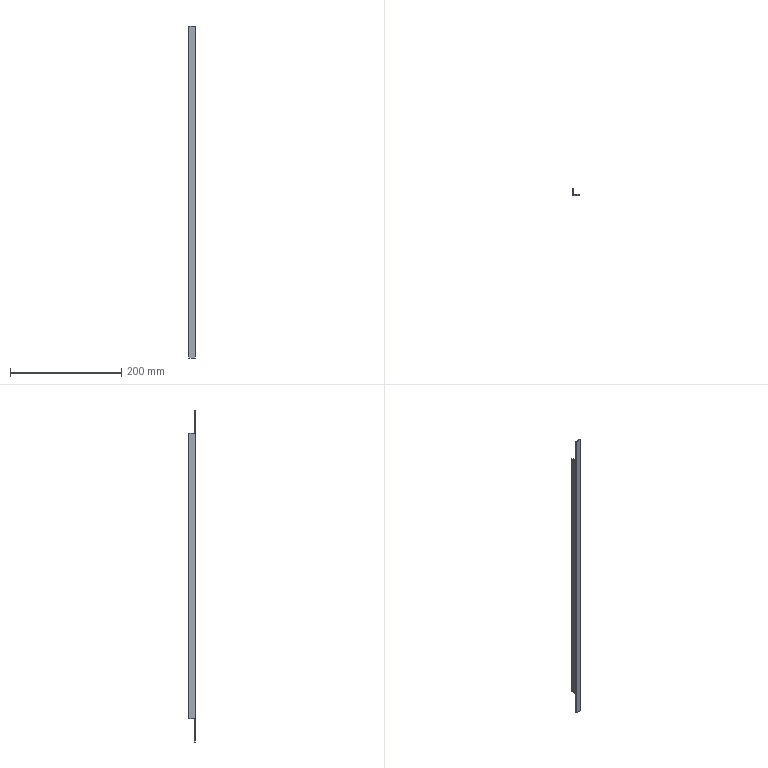Part | SolidWorks | features BaseBody 1 | 1 solid | 20 faces | box 12 x 12 x 597.2 mm | volume 15203 mm3 | plane 14 | cylinder 6 | commonest cylinder face diameters 0.6 x4 1 x2
STEP:
#1=CARTESIAN_POINT('',(0.5,0.,298.6));
#2=VERTEX_POINT('',#1);
#3=CARTESIAN_POINT('',(0.5,0.,-298.6));
#4=VERTEX_POINT('',#3);
#5=CARTESIAN_POINT('',(0.5,0.,0.));
#6=DIRECTION('',(0.,0.,-1.));
#7=VECTOR('',#6,1000.);
#8=LINE('',#5,#7);
#9=EDGE_CURVE('',#2,#4,#8,.T.);
#10=ORIENTED_EDGE('',*,*,#9,.F.);
#11=CARTESIAN_POINT('',(0.,0.5,298.6));
#12=VERTEX_POINT('',#11);
#13=CARTESIAN_POINT('',(0.5,0.5,298.6));
#14=DIRECTION('',(0.,0.,-1.));
#15=DIRECTION('',(0.,1.,0.));
#16=AXIS2_PLACEMENT_3D('',#13,#14,#15);
#17=CIRCLE('',#16,0.5);
#18=EDGE_CURVE('',#2,#12,#17,.T.);
#19=ORIENTED_EDGE('',*,*,#18,.T.);
#20=CARTESIAN_POINT('',(0.,0.5,-298.6));
#21=VERTEX_POINT('',#20);
#22=CARTESIAN_POINT('',(0.,0.5,0.));
#23=DIRECTION('',(0.,0.,1.));
#24=VECTOR('',#23,1000.);
#25=LINE('',#22,#24);
#26=EDGE_CURVE('',#21,#12,#25,.T.);
#27=ORIENTED_EDGE('',*,*,#26,.F.);
#28=CARTESIAN_POINT('',(0.5,0.5,-298.6));
#29=DIRECTION('',(0.,0.,-1.));
#30=DIRECTION('',(0.,1.,0.));
#31=AXIS2_PLACEMENT_3D('',#28,#29,#30);
#32=CIRCLE('',#31,0.5);
#33=EDGE_CURVE('',#4,#21,#32,.T.);
#34=ORIENTED_EDGE('',*,*,#33,.F.);
#35=EDGE_LOOP('',(#10,#19,#27,#34));
#36=FACE_OUTER_BOUND('',#35,.T.);
#37=CARTESIAN_POINT('',(0.5,0.5,298.6));
#38=DIRECTION('',(0.,0.,-1.));
#39=DIRECTION('',(0.,1.,0.));
#40=AXIS2_PLACEMENT_3D('',#37,#38,#39);
#41=CYLINDRICAL_SURFACE('',#40,0.5);
#42=ADVANCED_FACE('',(#36),#41,.T.);
#43=CARTESIAN_POINT('',(11.7,0.,298.6));
#44=VERTEX_POINT('',#43);
#45=CARTESIAN_POINT('',(11.7,0.,-298.6));
#46=VERTEX_POINT('',#45);
#47=CARTESIAN_POINT('',(11.7,0.,0.));
#48=DIRECTION('',(0.,0.,-1.));
#49=VECTOR('',#48,1000.);
#50=LINE('',#47,#49);
#51=EDGE_CURVE('',#44,#46,#50,.T.);
#52=ORIENTED_EDGE('',*,*,#51,.F.);
#53=CARTESIAN_POINT('',(6.1,0.,298.6));
#54=DIRECTION('',(1.,0.,0.));
#55=VECTOR('',#54,1000.);
#56=LINE('',#53,#55);
#57=EDGE_CURVE('',#2,#44,#56,.T.);
#58=ORIENTED_EDGE('',*,*,#57,.F.);
#59=ORIENTED_EDGE('',*,*,#9,.T.);
#60=CARTESIAN_POINT('',(6.1,0.,-298.6));
#61=DIRECTION('',(-1.,0.,0.));
#62=VECTOR('',#61,1000.);
#63=LINE('',#60,#62);
#64=EDGE_CURVE('',#46,#4,#63,.T.);
#65=ORIENTED_EDGE('',*,*,#64,.F.);
#66=EDGE_LOOP('',(#52,#58,#59,#65));
#67=FACE_OUTER_BOUND('',#66,.T.);
#68=CARTESIAN_POINT('',(0.5,0.,-298.6));
#69=DIRECTION('',(0.,1.,0.));
#70=DIRECTION('',(0.,0.,1.));
#71=AXIS2_PLACEMENT_3D('',#68,#69,#70);
#72=PLANE('',#71);
#73=ADVANCED_FACE('',(#67),#72,.F.);
#74=CARTESIAN_POINT('',(0.,1.2,-298.6));
#75=VERTEX_POINT('',#74);
#76=CARTESIAN_POINT('',(0.,1.2,-256.4));
#77=VERTEX_POINT('',#76);
#78=CARTESIAN_POINT('',(0.,1.2,0.));
#79=DIRECTION('',(0.,0.,1.));
#80=VECTOR('',#79,1000.);
#81=LINE('',#78,#80);
#82=EDGE_CURVE('',#75,#77,#81,.T.);
#83=ORIENTED_EDGE('',*,*,#82,.F.);
#84=CARTESIAN_POINT('',(0.,6.1,-298.6));
#85=DIRECTION('',(0.,1.,0.));
#86=VECTOR('',#85,1000.);
#87=LINE('',#84,#86);
#88=EDGE_CURVE('',#21,#75,#87,.T.);
#89=ORIENTED_EDGE('',*,*,#88,.F.);
#90=ORIENTED_EDGE('',*,*,#26,.T.);
#91=CARTESIAN_POINT('',(0.,1.2,298.6));
#92=VERTEX_POINT('',#91);
#93=CARTESIAN_POINT('',(0.,6.1,298.6));
#94=DIRECTION('',(0.,-1.,0.));
#95=VECTOR('',#94,1000.);
#96=LINE('',#93,#95);
#97=EDGE_CURVE('',#92,#12,#96,.T.);
#98=ORIENTED_EDGE('',*,*,#97,.F.);
#99=CARTESIAN_POINT('',(0.,1.2,256.4));
#100=VERTEX_POINT('',#99);
#101=CARTESIAN_POINT('',(0.,1.2,0.));
#102=DIRECTION('',(0.,0.,1.));
#103=VECTOR('',#102,1000.);
#104=LINE('',#101,#103);
#105=EDGE_CURVE('',#100,#92,#104,.T.);
#106=ORIENTED_EDGE('',*,*,#105,.F.);
#107=CARTESIAN_POINT('',(0.,11.7,256.4));
#108=VERTEX_POINT('',#107);
#109=CARTESIAN_POINT('',(0.,6.1,256.4));
#110=DIRECTION('',(0.,-1.,0.));
#111=VECTOR('',#110,1000.);
#112=LINE('',#109,#111);
#113=EDGE_CURVE('',#108,#100,#112,.T.);
#114=ORIENTED_EDGE('',*,*,#113,.F.);
#115=CARTESIAN_POINT('',(0.,11.7,-256.4));
#116=VERTEX_POINT('',#115);
#117=CARTESIAN_POINT('',(0.,11.7,0.));
#118=DIRECTION('',(0.,0.,1.));
#119=VECTOR('',#118,1000.);
#120=LINE('',#117,#119);
#121=EDGE_CURVE('',#116,#108,#120,.T.);
#122=ORIENTED_EDGE('',*,*,#121,.F.);
#123=CARTESIAN_POINT('',(0.,6.1,-256.4));
#124=DIRECTION('',(0.,1.,0.));
#125=VECTOR('',#124,1000.);
#126=LINE('',#123,#125);
#127=EDGE_CURVE('',#77,#116,#126,.T.);
#128=ORIENTED_EDGE('',*,*,#127,.F.);
#129=EDGE_LOOP('',(#83,#89,#90,#98,#106,#114,#122,#128));
#130=FACE_OUTER_BOUND('',#129,.T.);
#131=CARTESIAN_POINT('',(0.,0.5,298.6));
#132=DIRECTION('',(1.,0.,0.));
#133=DIRECTION('',(0.,0.,-1.));
#134=AXIS2_PLACEMENT_3D('',#131,#132,#133);
#135=PLANE('',#134);
#136=ADVANCED_FACE('',(#130),#135,.F.);
#137=ORIENTED_EDGE('',*,*,#33,.T.);
#138=ORIENTED_EDGE('',*,*,#88,.T.);
#139=CARTESIAN_POINT('',(1.2,1.2,-298.6));
#140=VERTEX_POINT('',#139);
#141=CARTESIAN_POINT('',(6.,1.2,-298.6));
#142=DIRECTION('',(1.,0.,0.));
#143=VECTOR('',#142,1000.);
#144=LINE('',#141,#143);
#145=EDGE_CURVE('',#75,#140,#144,.T.);
#146=ORIENTED_EDGE('',*,*,#145,.T.);
#147=CARTESIAN_POINT('',(1.2,1.7,-298.6));
#148=VERTEX_POINT('',#147);
#149=CARTESIAN_POINT('',(1.2,1.45,-298.6));
#150=DIRECTION('',(0.,1.,0.));
#151=VECTOR('',#150,1000.);
#152=LINE('',#149,#151);
#153=EDGE_CURVE('',#140,#148,#152,.T.);
#154=ORIENTED_EDGE('',*,*,#153,.T.);
#155=CARTESIAN_POINT('',(1.7,1.2,-298.6));
#156=VERTEX_POINT('',#155);
#157=CARTESIAN_POINT('',(1.7,1.7,-298.6));
#158=DIRECTION('',(0.,0.,-1.));
#159=DIRECTION('',(0.,1.,0.));
#160=AXIS2_PLACEMENT_3D('',#157,#158,#159);
#161=CIRCLE('',#160,0.5);
#162=EDGE_CURVE('',#156,#148,#161,.T.);
#163=ORIENTED_EDGE('',*,*,#162,.F.);
#164=CARTESIAN_POINT('',(11.7,1.2,-298.6));
#165=VERTEX_POINT('',#164);
#166=CARTESIAN_POINT('',(6.,1.2,-298.6));
#167=DIRECTION('',(1.,0.,0.));
#168=VECTOR('',#167,1000.);
#169=LINE('',#166,#168);
#170=EDGE_CURVE('',#156,#165,#169,.T.);
#171=ORIENTED_EDGE('',*,*,#170,.T.);
#172=CARTESIAN_POINT('',(12.,0.9,-298.6));
#173=VERTEX_POINT('',#172);
#174=CARTESIAN_POINT('',(11.7,0.9,-298.6));
#175=DIRECTION('',(0.,0.,-1.));
#176=DIRECTION('',(0.,1.,0.));
#177=AXIS2_PLACEMENT_3D('',#174,#175,#176);
#178=CIRCLE('',#177,0.3);
#179=EDGE_CURVE('',#165,#173,#178,.T.);
#180=ORIENTED_EDGE('',*,*,#179,.T.);
#181=CARTESIAN_POINT('',(12.,0.3,-298.6));
#182=VERTEX_POINT('',#181);
#183=CARTESIAN_POINT('',(12.,0.6,-298.6));
#184=DIRECTION('',(0.,-1.,0.));
#185=VECTOR('',#184,1000.);
#186=LINE('',#183,#185);
#187=EDGE_CURVE('',#173,#182,#186,.T.);
#188=ORIENTED_EDGE('',*,*,#187,.T.);
#189=CARTESIAN_POINT('',(11.7,0.3,-298.6));
#190=DIRECTION('',(0.,0.,-1.));
#191=DIRECTION('',(0.,1.,0.));
#192=AXIS2_PLACEMENT_3D('',#189,#190,#191);
#193=CIRCLE('',#192,0.3);
#194=EDGE_CURVE('',#182,#46,#193,.T.);
#195=ORIENTED_EDGE('',*,*,#194,.T.);
#196=ORIENTED_EDGE('',*,*,#64,.T.);
#197=EDGE_LOOP('',(#137,#138,#146,#154,#163,#171,#180,#188,#195,#196));
#198=FACE_OUTER_BOUND('',#197,.T.);
#199=CARTESIAN_POINT('',(12.,0.,-298.6));
#200=DIRECTION('',(0.,0.,-1.));
#201=DIRECTION('',(-1.,0.,0.));
#202=AXIS2_PLACEMENT_3D('',#199,#200,#201);
#203=PLANE('',#202);
#204=ADVANCED_FACE('',(#198),#203,.T.);
#205=CARTESIAN_POINT('',(12.,0.3,298.6));
#206=VERTEX_POINT('',#205);
#207=CARTESIAN_POINT('',(12.,0.3,0.));
#208=DIRECTION('',(0.,0.,-1.));
#209=VECTOR('',#208,1000.);
#210=LINE('',#207,#209);
#211=EDGE_CURVE('',#206,#182,#210,.T.);
#212=ORIENTED_EDGE('',*,*,#211,.F.);
#213=CARTESIAN_POINT('',(11.7,0.3,298.6));
#214=DIRECTION('',(0.,0.,1.));
#215=DIRECTION('',(0.,1.,0.));
#216=AXIS2_PLACEMENT_3D('',#213,#214,#215);
#217=CIRCLE('',#216,0.3);
#218=EDGE_CURVE('',#44,#206,#217,.T.);
#219=ORIENTED_EDGE('',*,*,#218,.F.);
#220=ORIENTED_EDGE('',*,*,#51,.T.);
#221=ORIENTED_EDGE('',*,*,#194,.F.);
#222=EDGE_LOOP('',(#212,#219,#220,#221));
#223=FACE_OUTER_BOUND('',#222,.T.);
#224=CARTESIAN_POINT('',(11.7,0.3,298.6));
#225=DIRECTION('',(0.,0.,-1.));
#226=DIRECTION('',(0.,1.,0.));
#227=AXIS2_PLACEMENT_3D('',#224,#225,#226);
#228=CYLINDRICAL_SURFACE('',#227,0.3);
#229=ADVANCED_FACE('',(#223),#228,.T.);
#230=CARTESIAN_POINT('',(1.2,1.2,298.6));
#231=VERTEX_POINT('',#230);
#232=CARTESIAN_POINT('',(6.,1.2,298.6));
#233=DIRECTION('',(1.,0.,0.));
#234=VECTOR('',#233,1000.);
#235=LINE('',#232,#234);
#236=EDGE_CURVE('',#92,#231,#235,.T.);
#237=ORIENTED_EDGE('',*,*,#236,.F.);
#238=ORIENTED_EDGE('',*,*,#97,.T.);
#239=ORIENTED_EDGE('',*,*,#18,.F.);
#240=ORIENTED_EDGE('',*,*,#57,.T.);
#241=ORIENTED_EDGE('',*,*,#218,.T.);
#242=CARTESIAN_POINT('',(12.,0.9,298.6));
#243=VERTEX_POINT('',#242);
#244=CARTESIAN_POINT('',(12.,0.8551,298.6));
#245=DIRECTION('',(0.,-1.,0.));
#246=VECTOR('',#245,1000.);
#247=LINE('',#244,#246);
#248=EDGE_CURVE('',#243,#206,#247,.T.);
#249=ORIENTED_EDGE('',*,*,#248,.F.);
#250=CARTESIAN_POINT('',(11.7,1.2,298.6));
#251=VERTEX_POINT('',#250);
#252=CARTESIAN_POINT('',(11.7,0.9,298.6));
#253=DIRECTION('',(0.,0.,1.));
#254=DIRECTION('',(0.,1.,0.));
#255=AXIS2_PLACEMENT_3D('',#252,#253,#254);
#256=CIRCLE('',#255,0.3);
#257=EDGE_CURVE('',#243,#251,#256,.T.);
#258=ORIENTED_EDGE('',*,*,#257,.T.);
#259=CARTESIAN_POINT('',(1.7,1.2,298.6));
#260=VERTEX_POINT('',#259);
#261=CARTESIAN_POINT('',(6.,1.2,298.6));
#262=DIRECTION('',(1.,0.,0.));
#263=VECTOR('',#262,1000.);
#264=LINE('',#261,#263);
#265=EDGE_CURVE('',#260,#251,#264,.T.);
#266=ORIENTED_EDGE('',*,*,#265,.F.);
#267=CARTESIAN_POINT('',(1.2,1.7,298.6));
#268=VERTEX_POINT('',#267);
#269=CARTESIAN_POINT('',(1.7,1.7,298.6));
#270=DIRECTION('',(0.,0.,1.));
#271=DIRECTION('',(0.,1.,0.));
#272=AXIS2_PLACEMENT_3D('',#269,#270,#271);
#273=CIRCLE('',#272,0.5);
#274=EDGE_CURVE('',#268,#260,#273,.T.);
#275=ORIENTED_EDGE('',*,*,#274,.F.);
#276=CARTESIAN_POINT('',(1.2,1.45,298.6));
#277=DIRECTION('',(0.,1.,0.));
#278=VECTOR('',#277,1000.);
#279=LINE('',#276,#278);
#280=EDGE_CURVE('',#231,#268,#279,.T.);
#281=ORIENTED_EDGE('',*,*,#280,.F.);
#282=EDGE_LOOP('',(#237,#238,#239,#240,#241,#249,#258,#266,#275,#281));
#283=FACE_OUTER_BOUND('',#282,.T.);
#284=CARTESIAN_POINT('',(12.,0.,298.6));
#285=DIRECTION('',(0.,0.,-1.));
#286=DIRECTION('',(-1.,0.,0.));
#287=AXIS2_PLACEMENT_3D('',#284,#285,#286);
#288=PLANE('',#287);
#289=ADVANCED_FACE('',(#283),#288,.F.);
#290=CARTESIAN_POINT('',(1.2,1.7,-256.4));
#291=VERTEX_POINT('',#290);
#292=CARTESIAN_POINT('',(1.2,1.2,-256.4));
#293=VERTEX_POINT('',#292);
#294=CARTESIAN_POINT('',(1.2,1.45,-256.4));
#295=DIRECTION('',(0.,-1.,0.));
#296=VECTOR('',#295,1000.);
#297=LINE('',#294,#296);
#298=EDGE_CURVE('',#291,#293,#297,.T.);
#299=ORIENTED_EDGE('',*,*,#298,.T.);
#300=CARTESIAN_POINT('',(0.6,1.2,-256.4));
#301=DIRECTION('',(1.,0.,0.));
#302=VECTOR('',#301,1000.);
#303=LINE('',#300,#302);
#304=EDGE_CURVE('',#77,#293,#303,.T.);
#305=ORIENTED_EDGE('',*,*,#304,.F.);
#306=ORIENTED_EDGE('',*,*,#127,.T.);
#307=CARTESIAN_POINT('',(0.3,12.,-256.4));
#308=VERTEX_POINT('',#307);
#309=CARTESIAN_POINT('',(0.3,11.7,-256.4));
#310=DIRECTION('',(0.,0.,1.));
#311=DIRECTION('',(-1.,0.,0.));
#312=AXIS2_PLACEMENT_3D('',#309,#310,#311);
#313=CIRCLE('',#312,0.3);
#314=EDGE_CURVE('',#308,#116,#313,.T.);
#315=ORIENTED_EDGE('',*,*,#314,.F.);
#316=CARTESIAN_POINT('',(0.9,12.,-256.4));
#317=VERTEX_POINT('',#316);
#318=CARTESIAN_POINT('',(0.6,12.,-256.4));
#319=DIRECTION('',(1.,0.,0.));
#320=VECTOR('',#319,1000.);
#321=LINE('',#318,#320);
#322=EDGE_CURVE('',#308,#317,#321,.T.);
#323=ORIENTED_EDGE('',*,*,#322,.T.);
#324=CARTESIAN_POINT('',(1.2,11.7,-256.4));
#325=VERTEX_POINT('',#324);
#326=CARTESIAN_POINT('',(0.9,11.7,-256.4));
#327=DIRECTION('',(0.,0.,-1.));
#328=DIRECTION('',(-1.,0.,0.));
#329=AXIS2_PLACEMENT_3D('',#326,#327,#328);
#330=CIRCLE('',#329,0.3);
#331=EDGE_CURVE('',#317,#325,#330,.T.);
#332=ORIENTED_EDGE('',*,*,#331,.T.);
#333=CARTESIAN_POINT('',(1.2,6.6,-256.4));
#334=DIRECTION('',(0.,1.,0.));
#335=VECTOR('',#334,1000.);
#336=LINE('',#333,#335);
#337=EDGE_CURVE('',#291,#325,#336,.T.);
#338=ORIENTED_EDGE('',*,*,#337,.F.);
#339=EDGE_LOOP('',(#299,#305,#306,#315,#323,#332,#338));
#340=FACE_OUTER_BOUND('',#339,.T.);
#341=CARTESIAN_POINT('',(0.,1.2,-256.4));
#342=DIRECTION('',(0.,0.,1.));
#343=DIRECTION('',(1.,0.,0.));
#344=AXIS2_PLACEMENT_3D('',#341,#342,#343);
#345=PLANE('',#344);
#346=ADVANCED_FACE('',(#340),#345,.F.);
#347=CARTESIAN_POINT('',(1.2,1.2,-277.5));
#348=DIRECTION('',(0.,0.,1.));
#349=VECTOR('',#348,1000.);
#350=LINE('',#347,#349);
#351=EDGE_CURVE('',#140,#293,#350,.T.);
#352=ORIENTED_EDGE('',*,*,#351,.F.);
#353=ORIENTED_EDGE('',*,*,#145,.F.);
#354=ORIENTED_EDGE('',*,*,#82,.T.);
#355=ORIENTED_EDGE('',*,*,#304,.T.);
#356=EDGE_LOOP('',(#352,#353,#354,#355));
#357=FACE_OUTER_BOUND('',#356,.T.);
#358=CARTESIAN_POINT('',(0.,1.2,-298.6));
#359=DIRECTION('',(0.,-1.,0.));
#360=DIRECTION('',(1.,0.,0.));
#361=AXIS2_PLACEMENT_3D('',#358,#359,#360);
#362=PLANE('',#361);
#363=ADVANCED_FACE('',(#357),#362,.F.);
#364=CARTESIAN_POINT('',(1.2,1.2,256.4));
#365=VERTEX_POINT('',#364);
#366=CARTESIAN_POINT('',(1.2,1.2,277.5));
#367=DIRECTION('',(0.,0.,1.));
#368=VECTOR('',#367,1000.);
#369=LINE('',#366,#368);
#370=EDGE_CURVE('',#365,#231,#369,.T.);
#371=ORIENTED_EDGE('',*,*,#370,.F.);
#372=CARTESIAN_POINT('',(0.6,1.2,256.4));
#373=DIRECTION('',(1.,0.,0.));
#374=VECTOR('',#373,1000.);
#375=LINE('',#372,#374);
#376=EDGE_CURVE('',#100,#365,#375,.T.);
#377=ORIENTED_EDGE('',*,*,#376,.F.);
#378=ORIENTED_EDGE('',*,*,#105,.T.);
#379=ORIENTED_EDGE('',*,*,#236,.T.);
#380=EDGE_LOOP('',(#371,#377,#378,#379));
#381=FACE_OUTER_BOUND('',#380,.T.);
#382=CARTESIAN_POINT('',(0.,1.2,256.4));
#383=DIRECTION('',(0.,-1.,0.));
#384=DIRECTION('',(1.,0.,0.));
#385=AXIS2_PLACEMENT_3D('',#382,#383,#384);
#386=PLANE('',#385);
#387=ADVANCED_FACE('',(#381),#386,.F.);
#388=CARTESIAN_POINT('',(0.3,12.,256.4));
#389=VERTEX_POINT('',#388);
#390=CARTESIAN_POINT('',(0.3,11.7,256.4));
#391=DIRECTION('',(0.,0.,-1.));
#392=DIRECTION('',(-1.,0.,0.));
#393=AXIS2_PLACEMENT_3D('',#390,#391,#392);
#394=CIRCLE('',#393,0.3);
#395=EDGE_CURVE('',#108,#389,#394,.T.);
#396=ORIENTED_EDGE('',*,*,#395,.F.);
#397=ORIENTED_EDGE('',*,*,#113,.T.);
#398=ORIENTED_EDGE('',*,*,#376,.T.);
#399=CARTESIAN_POINT('',(1.2,1.7,256.4));
#400=VERTEX_POINT('',#399);
#401=CARTESIAN_POINT('',(1.2,6.6,256.4));
#402=DIRECTION('',(0.,-1.,0.));
#403=VECTOR('',#402,1000.);
#404=LINE('',#401,#403);
#405=EDGE_CURVE('',#400,#365,#404,.T.);
#406=ORIENTED_EDGE('',*,*,#405,.F.);
#407=CARTESIAN_POINT('',(1.2,11.7,256.4));
#408=VERTEX_POINT('',#407);
#409=CARTESIAN_POINT('',(1.2,6.6,256.4));
#410=DIRECTION('',(0.,-1.,0.));
#411=VECTOR('',#410,1000.);
#412=LINE('',#409,#411);
#413=EDGE_CURVE('',#408,#400,#412,.T.);
#414=ORIENTED_EDGE('',*,*,#413,.F.);
#415=CARTESIAN_POINT('',(0.9,12.,256.4));
#416=VERTEX_POINT('',#415);
#417=CARTESIAN_POINT('',(0.9,11.7,256.4));
#418=DIRECTION('',(0.,0.,1.));
#419=DIRECTION('',(-1.,0.,0.));
#420=AXIS2_PLACEMENT_3D('',#417,#418,#419);
#421=CIRCLE('',#420,0.3);
#422=EDGE_CURVE('',#408,#416,#421,.T.);
#423=ORIENTED_EDGE('',*,*,#422,.T.);
#424=CARTESIAN_POINT('',(0.6,12.,256.4));
#425=DIRECTION('',(-1.,0.,0.));
#426=VECTOR('',#425,1000.);
#427=LINE('',#424,#426);
#428=EDGE_CURVE('',#416,#389,#427,.T.);
#429=ORIENTED_EDGE('',*,*,#428,.T.);
#430=EDGE_LOOP('',(#396,#397,#398,#406,#414,#423,#429));
#431=FACE_OUTER_BOUND('',#430,.T.);
#432=CARTESIAN_POINT('',(1.2,1.2,256.4));
#433=DIRECTION('',(0.,0.,-1.));
#434=DIRECTION('',(-1.,0.,0.));
#435=AXIS2_PLACEMENT_3D('',#432,#433,#434);
#436=PLANE('',#435);
#437=ADVANCED_FACE('',(#431),#436,.F.);
#438=ORIENTED_EDGE('',*,*,#314,.T.);
#439=ORIENTED_EDGE('',*,*,#121,.T.);
#440=ORIENTED_EDGE('',*,*,#395,.T.);
#441=CARTESIAN_POINT('',(0.3,12.,0.));
#442=DIRECTION('',(0.,0.,1.));
#443=VECTOR('',#442,1000.);
#444=LINE('',#441,#443);
#445=EDGE_CURVE('',#308,#389,#444,.T.);
#446=ORIENTED_EDGE('',*,*,#445,.F.);
#447=EDGE_LOOP('',(#438,#439,#440,#446));
#448=FACE_OUTER_BOUND('',#447,.T.);
#449=CARTESIAN_POINT('',(0.3,11.7,256.4));
#450=DIRECTION('',(0.,0.,-1.));
#451=DIRECTION('',(-1.,0.,0.));
#452=AXIS2_PLACEMENT_3D('',#449,#450,#451);
#453=CYLINDRICAL_SURFACE('',#452,0.3);
#454=ADVANCED_FACE('',(#448),#453,.T.);
#455=CARTESIAN_POINT('',(1.7,1.2,0.));
#456=DIRECTION('',(0.,0.,-1.));
#457=VECTOR('',#456,1000.);
#458=LINE('',#455,#457);
#459=EDGE_CURVE('',#260,#156,#458,.T.);
#460=ORIENTED_EDGE('',*,*,#459,.F.);
#461=ORIENTED_EDGE('',*,*,#265,.T.);
#462=CARTESIAN_POINT('',(11.7,1.2,0.));
#463=DIRECTION('',(0.,0.,1.));
#464=VECTOR('',#463,1000.);
#465=LINE('',#462,#464);
#466=EDGE_CURVE('',#165,#251,#465,.T.);
#467=ORIENTED_EDGE('',*,*,#466,.F.);
#468=ORIENTED_EDGE('',*,*,#170,.F.);
#469=EDGE_LOOP('',(#460,#461,#467,#468));
#470=FACE_OUTER_BOUND('',#469,.T.);
#471=CARTESIAN_POINT('',(1.7,1.2,-298.6));
#472=DIRECTION('',(0.,-1.,0.));
#473=DIRECTION('',(1.,0.,0.));
#474=AXIS2_PLACEMENT_3D('',#471,#472,#473);
#475=PLANE('',#474);
#476=ADVANCED_FACE('',(#470),#475,.F.);
#477=CARTESIAN_POINT('',(12.,0.9,0.));
#478=DIRECTION('',(0.,0.,-1.));
#479=VECTOR('',#478,1000.);
#480=LINE('',#477,#479);
#481=EDGE_CURVE('',#243,#173,#480,.T.);
#482=ORIENTED_EDGE('',*,*,#481,.F.);
#483=ORIENTED_EDGE('',*,*,#248,.T.);
#484=ORIENTED_EDGE('',*,*,#211,.T.);
#485=ORIENTED_EDGE('',*,*,#187,.F.);
#486=EDGE_LOOP('',(#482,#483,#484,#485));
#487=FACE_OUTER_BOUND('',#486,.T.);
#488=CARTESIAN_POINT('',(12.,0.3,-298.6));
#489=DIRECTION('',(-1.,0.,0.));
#490=DIRECTION('',(0.,0.,1.));
#491=AXIS2_PLACEMENT_3D('',#488,#489,#490);
#492=PLANE('',#491);
#493=ADVANCED_FACE('',(#487),#492,.F.);
#494=ORIENTED_EDGE('',*,*,#337,.T.);
#495=CARTESIAN_POINT('',(1.2,11.7,0.));
#496=DIRECTION('',(0.,0.,-1.));
#497=VECTOR('',#496,1000.);
#498=LINE('',#495,#497);
#499=EDGE_CURVE('',#408,#325,#498,.T.);
#500=ORIENTED_EDGE('',*,*,#499,.F.);
#501=ORIENTED_EDGE('',*,*,#413,.T.);
#502=CARTESIAN_POINT('',(1.2,1.7,0.));
#503=DIRECTION('',(0.,0.,1.));
#504=VECTOR('',#503,1000.);
#505=LINE('',#502,#504);
#506=EDGE_CURVE('',#291,#400,#505,.T.);
#507=ORIENTED_EDGE('',*,*,#506,.F.);
#508=EDGE_LOOP('',(#494,#500,#501,#507));
#509=FACE_OUTER_BOUND('',#508,.T.);
#510=CARTESIAN_POINT('',(1.2,11.7,-256.4));
#511=DIRECTION('',(-1.,0.,0.));
#512=DIRECTION('',(0.,-1.,0.));
#513=AXIS2_PLACEMENT_3D('',#510,#511,#512);
#514=PLANE('',#513);
#515=ADVANCED_FACE('',(#509),#514,.F.);
#516=ORIENTED_EDGE('',*,*,#351,.T.);
#517=ORIENTED_EDGE('',*,*,#298,.F.);
#518=CARTESIAN_POINT('',(1.2,1.7,-277.5));
#519=DIRECTION('',(0.,0.,1.));
#520=VECTOR('',#519,1000.);
#521=LINE('',#518,#520);
#522=EDGE_CURVE('',#148,#291,#521,.T.);
#523=ORIENTED_EDGE('',*,*,#522,.F.);
#524=ORIENTED_EDGE('',*,*,#153,.F.);
#525=EDGE_LOOP('',(#516,#517,#523,#524));
#526=FACE_OUTER_BOUND('',#525,.T.);
#527=CARTESIAN_POINT('',(1.2,1.2,-298.6));
#528=DIRECTION('',(1.,0.,0.));
#529=DIRECTION('',(0.,1.,0.));
#530=AXIS2_PLACEMENT_3D('',#527,#528,#529);
#531=PLANE('',#530);
#532=ADVANCED_FACE('',(#526),#531,.F.);
#533=ORIENTED_EDGE('',*,*,#280,.T.);
#534=CARTESIAN_POINT('',(1.2,1.7,277.5));
#535=DIRECTION('',(0.,0.,-1.));
#536=VECTOR('',#535,1000.);
#537=LINE('',#534,#536);
#538=EDGE_CURVE('',#268,#400,#537,.T.);
#539=ORIENTED_EDGE('',*,*,#538,.T.);
#540=ORIENTED_EDGE('',*,*,#405,.T.);
#541=ORIENTED_EDGE('',*,*,#370,.T.);
#542=EDGE_LOOP('',(#533,#539,#540,#541));
#543=FACE_OUTER_BOUND('',#542,.T.);
#544=CARTESIAN_POINT('',(1.2,1.7,256.4));
#545=DIRECTION('',(-1.,0.,0.));
#546=DIRECTION('',(0.,-1.,0.));
#547=AXIS2_PLACEMENT_3D('',#544,#545,#546);
#548=PLANE('',#547);
#549=ADVANCED_FACE('',(#543),#548,.T.);
#550=ORIENTED_EDGE('',*,*,#322,.F.);
#551=ORIENTED_EDGE('',*,*,#445,.T.);
#552=ORIENTED_EDGE('',*,*,#428,.F.);
#553=CARTESIAN_POINT('',(0.9,12.,0.));
#554=DIRECTION('',(0.,0.,1.));
#555=VECTOR('',#554,1000.);
#556=LINE('',#553,#555);
#557=EDGE_CURVE('',#317,#416,#556,.T.);
#558=ORIENTED_EDGE('',*,*,#557,.F.);
#559=EDGE_LOOP('',(#550,#551,#552,#558));
#560=FACE_OUTER_BOUND('',#559,.T.);
#561=CARTESIAN_POINT('',(0.3,12.,256.4));
#562=DIRECTION('',(0.,-1.,0.));
#563=DIRECTION('',(0.,0.,-1.));
#564=AXIS2_PLACEMENT_3D('',#561,#562,#563);
#565=PLANE('',#564);
#566=ADVANCED_FACE('',(#560),#565,.F.);
#567=ORIENTED_EDGE('',*,*,#274,.T.);
#568=ORIENTED_EDGE('',*,*,#459,.T.);
#569=ORIENTED_EDGE('',*,*,#162,.T.);
#570=ORIENTED_EDGE('',*,*,#522,.T.);
#571=ORIENTED_EDGE('',*,*,#506,.T.);
#572=ORIENTED_EDGE('',*,*,#538,.F.);
#573=EDGE_LOOP('',(#567,#568,#569,#570,#571,#572));
#574=FACE_OUTER_BOUND('',#573,.T.);
#575=CARTESIAN_POINT('',(1.7,1.7,298.6));
#576=DIRECTION('',(0.,0.,-1.));
#577=DIRECTION('',(0.,1.,0.));
#578=AXIS2_PLACEMENT_3D('',#575,#576,#577);
#579=CYLINDRICAL_SURFACE('',#578,0.5);
#580=ADVANCED_FACE('',(#574),#579,.F.);
#581=ORIENTED_EDGE('',*,*,#466,.T.);
#582=ORIENTED_EDGE('',*,*,#257,.F.);
#583=ORIENTED_EDGE('',*,*,#481,.T.);
#584=ORIENTED_EDGE('',*,*,#179,.F.);
#585=EDGE_LOOP('',(#581,#582,#583,#584));
#586=FACE_OUTER_BOUND('',#585,.T.);
#587=CARTESIAN_POINT('',(11.7,0.9,298.6));
#588=DIRECTION('',(0.,0.,-1.));
#589=DIRECTION('',(0.,1.,0.));
#590=AXIS2_PLACEMENT_3D('',#587,#588,#589);
#591=CYLINDRICAL_SURFACE('',#590,0.3);
#592=ADVANCED_FACE('',(#586),#591,.T.);
#593=ORIENTED_EDGE('',*,*,#331,.F.);
#594=ORIENTED_EDGE('',*,*,#557,.T.);
#595=ORIENTED_EDGE('',*,*,#422,.F.);
#596=ORIENTED_EDGE('',*,*,#499,.T.);
#597=EDGE_LOOP('',(#593,#594,#595,#596));
#598=FACE_OUTER_BOUND('',#597,.T.);
#599=CARTESIAN_POINT('',(0.9,11.7,256.4));
#600=DIRECTION('',(0.,0.,-1.));
#601=DIRECTION('',(-1.,0.,0.));
#602=AXIS2_PLACEMENT_3D('',#599,#600,#601);
#603=CYLINDRICAL_SURFACE('',#602,0.3);
#604=ADVANCED_FACE('',(#598),#603,.T.);
#605=CLOSED_SHELL('',(#42,#73,#136,#204,#229,#289,#346,#363,#387,#437,#454,#476,#493,#515,#532,#549,#566,#580,#592,#604));
#606=MANIFOLD_SOLID_BREP('',#605);
#607=CARTESIAN_POINT('',(0.,0.,0.));
#608=DIRECTION('',(0.,0.,1.));
#609=DIRECTION('',(1.,0.,0.));
#610=AXIS2_PLACEMENT_3D('',#607,#608,#609);
#611=(LENGTH_UNIT()NAMED_UNIT(*)SI_UNIT(.MILLI.,.METRE.));
#612=UNCERTAINTY_MEASURE_WITH_UNIT(LENGTH_MEASURE(0.00001),#611,'','');
#613=(NAMED_UNIT(*)PLANE_ANGLE_UNIT()SI_UNIT($,.RADIAN.));
#614=(NAMED_UNIT(*)SI_UNIT($,.STERADIAN.)SOLID_ANGLE_UNIT());
#615=(GEOMETRIC_REPRESENTATION_CONTEXT(3)GLOBAL_UNCERTAINTY_ASSIGNED_CONTEXT((#612))GLOBAL_UNIT_ASSIGNED_CONTEXT((#611,#613,#614))REPRESENTATION_CONTEXT('',''));
#616=ADVANCED_BREP_SHAPE_REPRESENTATION('',(#606,#610),#615);